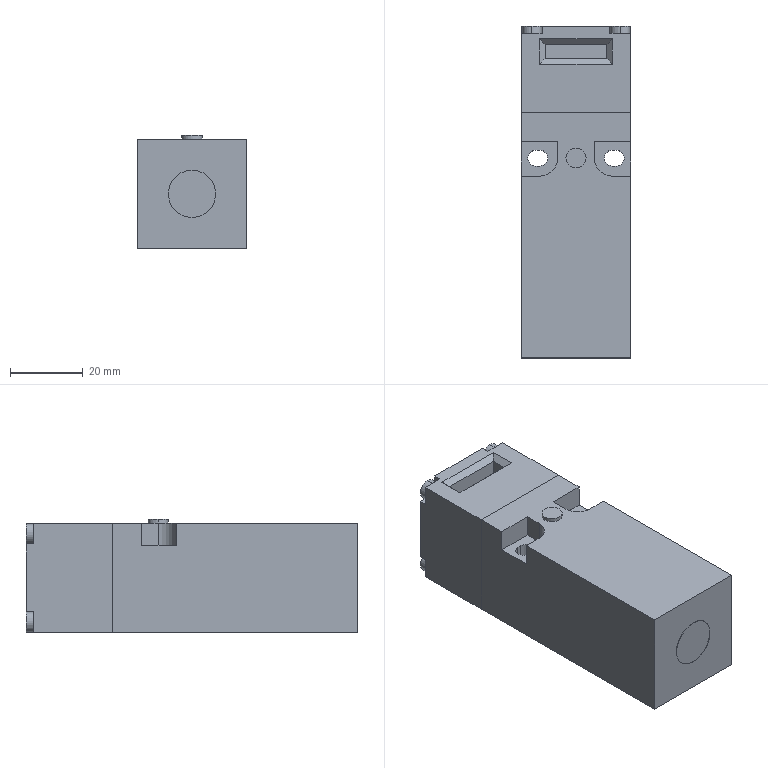Part | SolidWorks | features BaseBody 2 | 2 solids | 108 faces | box 30 x 91 x 31 mm | volume 76497 mm3 | plane 70 | cylinder 38 | commonest cylinder face diameters 3 x16 5.5 x10 4.4 x4 5.6 x4 10 x2 13 x2